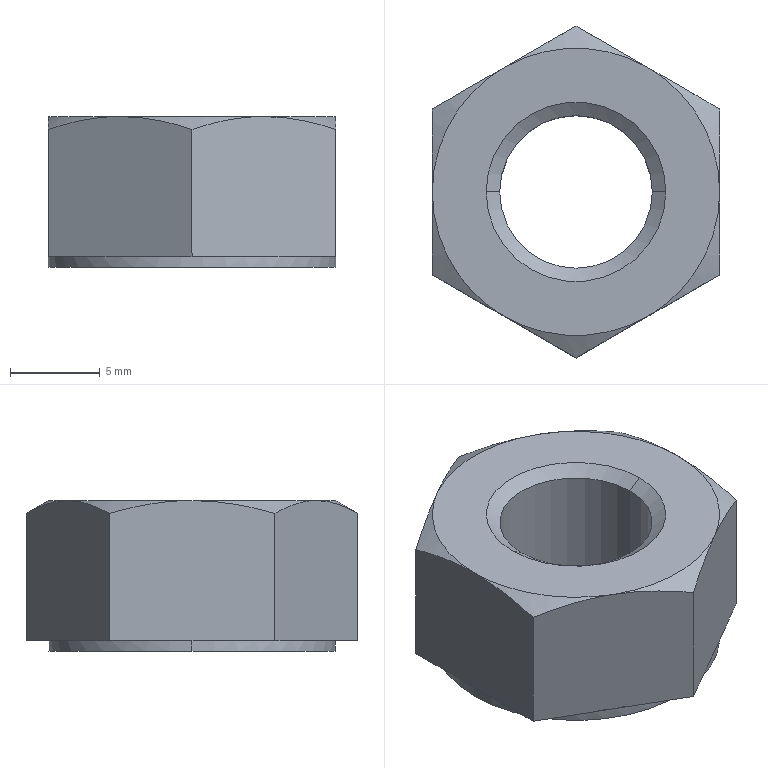Part | STEP file | hex nut style 1 gradeab_iso_ISO - 4032 - M10 - W - N | 1 solid | 30 faces | box 16 x 18.475 x 8.4 mm | volume 1357 mm3 | plane 14 | cone 10 | cylinder 6 | commonest cylinder face diameters 8.5 x2 10 x2 16 x2
STEP:
#1=CARTESIAN_POINT('',(5.,0.,-8.4));
#2=VERTEX_POINT('',#1);
#3=CARTESIAN_POINT('',(-5.,0.,-8.4));
#4=VERTEX_POINT('',#3);
#5=CARTESIAN_POINT('',(0.,0.,-8.4));
#6=DIRECTION('',(0.,0.,-1.));
#7=DIRECTION('',(1.,0.,0.));
#8=AXIS2_PLACEMENT_3D('',#5,#6,#7);
#9=CIRCLE('',#8,5.);
#10=EDGE_CURVE('',#2,#4,#9,.T.);
#11=ORIENTED_EDGE('',*,*,#10,.T.);
#12=CARTESIAN_POINT('',(-5.,0.,-8.375));
#13=VERTEX_POINT('',#12);
#14=CARTESIAN_POINT('',(-5.,0.,-25.038));
#15=DIRECTION('',(0.,0.,1.));
#16=VECTOR('',#15,1000.);
#17=LINE('',#14,#16);
#18=EDGE_CURVE('',#4,#13,#17,.T.);
#19=ORIENTED_EDGE('',*,*,#18,.T.);
#20=CARTESIAN_POINT('',(5.,0.,-8.375));
#21=VERTEX_POINT('',#20);
#22=CARTESIAN_POINT('',(0.,0.,-8.375));
#23=DIRECTION('',(0.,0.,1.));
#24=DIRECTION('',(1.,0.,0.));
#25=AXIS2_PLACEMENT_3D('',#22,#23,#24);
#26=CIRCLE('',#25,5.);
#27=EDGE_CURVE('',#13,#21,#26,.T.);
#28=ORIENTED_EDGE('',*,*,#27,.T.);
#29=CARTESIAN_POINT('',(5.,0.,-25.038));
#30=DIRECTION('',(0.,0.,1.));
#31=VECTOR('',#30,1000.);
#32=LINE('',#29,#31);
#33=EDGE_CURVE('',#2,#21,#32,.T.);
#34=ORIENTED_EDGE('',*,*,#33,.F.);
#35=EDGE_LOOP('',(#11,#19,#28,#34));
#36=FACE_OUTER_BOUND('',#35,.T.);
#37=CARTESIAN_POINT('',(0.,0.,-25.038));
#38=DIRECTION('',(0.,0.,1.));
#39=DIRECTION('',(1.,0.,0.));
#40=AXIS2_PLACEMENT_3D('',#37,#38,#39);
#41=CYLINDRICAL_SURFACE('',#40,5.);
#42=ADVANCED_FACE('',(#36),#41,.F.);
#43=CARTESIAN_POINT('',(-4.25,0.,-7.849));
#44=VERTEX_POINT('',#43);
#45=CARTESIAN_POINT('',(4.25,0.,-7.849));
#46=VERTEX_POINT('',#45);
#47=CARTESIAN_POINT('',(0.,0.,-7.849));
#48=DIRECTION('',(0.,0.,1.));
#49=DIRECTION('',(-1.,0.,0.));
#50=AXIS2_PLACEMENT_3D('',#47,#48,#49);
#51=CIRCLE('',#50,4.25);
#52=EDGE_CURVE('',#44,#46,#51,.T.);
#53=ORIENTED_EDGE('',*,*,#52,.T.);
#54=CARTESIAN_POINT('',(5.,0.,-8.375));
#55=DIRECTION('',(0.8192,0.,-0.5736));
#56=VECTOR('',#55,1000.);
#57=LINE('',#54,#56);
#58=EDGE_CURVE('',#46,#21,#57,.T.);
#59=ORIENTED_EDGE('',*,*,#58,.T.);
#60=ORIENTED_EDGE('',*,*,#27,.F.);
#61=CARTESIAN_POINT('',(-5.,0.,-8.375));
#62=DIRECTION('',(-0.8192,0.,-0.5736));
#63=VECTOR('',#62,1000.);
#64=LINE('',#61,#63);
#65=EDGE_CURVE('',#44,#13,#64,.T.);
#66=ORIENTED_EDGE('',*,*,#65,.F.);
#67=EDGE_LOOP('',(#53,#59,#60,#66));
#68=FACE_OUTER_BOUND('',#67,.T.);
#69=CARTESIAN_POINT('',(0.,0.,-8.375));
#70=DIRECTION('',(0.,0.,-1.));
#71=DIRECTION('',(-1.,0.,0.));
#72=AXIS2_PLACEMENT_3D('',#69,#70,#71);
#73=CONICAL_SURFACE('',#72,5.,0.9599);
#74=ADVANCED_FACE('',(#68),#73,.F.);
#75=CARTESIAN_POINT('',(4.25,0.,-0.5252));
#76=VERTEX_POINT('',#75);
#77=CARTESIAN_POINT('',(-4.25,0.,-0.5252));
#78=VERTEX_POINT('',#77);
#79=CARTESIAN_POINT('',(0.,0.,-0.5252));
#80=DIRECTION('',(0.,0.,-1.));
#81=DIRECTION('',(1.,0.,0.));
#82=AXIS2_PLACEMENT_3D('',#79,#80,#81);
#83=CIRCLE('',#82,4.25);
#84=EDGE_CURVE('',#76,#78,#83,.T.);
#85=ORIENTED_EDGE('',*,*,#84,.T.);
#86=CARTESIAN_POINT('',(-5.,0.,0.));
#87=VERTEX_POINT('',#86);
#88=CARTESIAN_POINT('',(-4.175,0.,-0.5777));
#89=DIRECTION('',(-0.8192,0.,0.5736));
#90=VECTOR('',#89,1000.);
#91=LINE('',#88,#90);
#92=EDGE_CURVE('',#78,#87,#91,.T.);
#93=ORIENTED_EDGE('',*,*,#92,.T.);
#94=CARTESIAN_POINT('',(5.,0.,0.));
#95=VERTEX_POINT('',#94);
#96=CARTESIAN_POINT('',(0.,0.,0.));
#97=DIRECTION('',(0.,0.,1.));
#98=DIRECTION('',(1.,0.,0.));
#99=AXIS2_PLACEMENT_3D('',#96,#97,#98);
#100=CIRCLE('',#99,5.);
#101=EDGE_CURVE('',#87,#95,#100,.T.);
#102=ORIENTED_EDGE('',*,*,#101,.T.);
#103=CARTESIAN_POINT('',(4.175,0.,-0.5777));
#104=DIRECTION('',(0.8192,0.,0.5736));
#105=VECTOR('',#104,1000.);
#106=LINE('',#103,#105);
#107=EDGE_CURVE('',#76,#95,#106,.T.);
#108=ORIENTED_EDGE('',*,*,#107,.F.);
#109=EDGE_LOOP('',(#85,#93,#102,#108));
#110=FACE_OUTER_BOUND('',#109,.T.);
#111=CARTESIAN_POINT('',(0.,0.,-0.5777));
#112=DIRECTION('',(0.,0.,1.));
#113=DIRECTION('',(1.,0.,0.));
#114=AXIS2_PLACEMENT_3D('',#111,#112,#113);
#115=CONICAL_SURFACE('',#114,4.175,0.9599);
#116=ADVANCED_FACE('',(#110),#115,.F.);
#117=CARTESIAN_POINT('',(-8.,0.,-8.4));
#118=VERTEX_POINT('',#117);
#119=CARTESIAN_POINT('',(8.,0.,-8.4));
#120=VERTEX_POINT('',#119);
#121=CARTESIAN_POINT('',(0.,0.,-8.4));
#122=DIRECTION('',(0.,0.,-1.));
#123=DIRECTION('',(1.,0.,0.));
#124=AXIS2_PLACEMENT_3D('',#121,#122,#123);
#125=CIRCLE('',#124,8.);
#126=EDGE_CURVE('',#118,#120,#125,.T.);
#127=ORIENTED_EDGE('',*,*,#126,.F.);
#128=CARTESIAN_POINT('',(-8.,0.,-7.8));
#129=VERTEX_POINT('',#128);
#130=CARTESIAN_POINT('',(-8.,0.,0.));
#131=DIRECTION('',(0.,0.,1.));
#132=VECTOR('',#131,1000.);
#133=LINE('',#130,#132);
#134=EDGE_CURVE('',#118,#129,#133,.T.);
#135=ORIENTED_EDGE('',*,*,#134,.T.);
#136=CARTESIAN_POINT('',(-4.,6.928,-7.8));
#137=VERTEX_POINT('',#136);
#138=CARTESIAN_POINT('',(0.,0.,-7.8));
#139=DIRECTION('',(0.,0.,1.));
#140=DIRECTION('',(1.,0.,0.));
#141=AXIS2_PLACEMENT_3D('',#138,#139,#140);
#142=CIRCLE('',#141,8.);
#143=EDGE_CURVE('',#137,#129,#142,.T.);
#144=ORIENTED_EDGE('',*,*,#143,.F.);
#145=CARTESIAN_POINT('',(4.,6.928,-7.8));
#146=VERTEX_POINT('',#145);
#147=CARTESIAN_POINT('',(0.,0.,-7.8));
#148=DIRECTION('',(0.,0.,1.));
#149=DIRECTION('',(1.,0.,0.));
#150=AXIS2_PLACEMENT_3D('',#147,#148,#149);
#151=CIRCLE('',#150,8.);
#152=EDGE_CURVE('',#146,#137,#151,.T.);
#153=ORIENTED_EDGE('',*,*,#152,.F.);
#154=CARTESIAN_POINT('',(8.,0.,-7.8));
#155=VERTEX_POINT('',#154);
#156=CARTESIAN_POINT('',(0.,0.,-7.8));
#157=DIRECTION('',(0.,0.,1.));
#158=DIRECTION('',(1.,0.,0.));
#159=AXIS2_PLACEMENT_3D('',#156,#157,#158);
#160=CIRCLE('',#159,8.);
#161=EDGE_CURVE('',#155,#146,#160,.T.);
#162=ORIENTED_EDGE('',*,*,#161,.F.);
#163=CARTESIAN_POINT('',(8.,0.,0.));
#164=DIRECTION('',(0.,0.,1.));
#165=VECTOR('',#164,1000.);
#166=LINE('',#163,#165);
#167=EDGE_CURVE('',#120,#155,#166,.T.);
#168=ORIENTED_EDGE('',*,*,#167,.F.);
#169=EDGE_LOOP('',(#127,#135,#144,#153,#162,#168));
#170=FACE_OUTER_BOUND('',#169,.T.);
#171=CARTESIAN_POINT('',(0.,0.,0.));
#172=DIRECTION('',(0.,0.,1.));
#173=DIRECTION('',(1.,0.,0.));
#174=AXIS2_PLACEMENT_3D('',#171,#172,#173);
#175=CYLINDRICAL_SURFACE('',#174,8.);
#176=ADVANCED_FACE('',(#170),#175,.T.);
#177=ORIENTED_EDGE('',*,*,#52,.F.);
#178=CARTESIAN_POINT('',(-4.25,0.,-8.4));
#179=DIRECTION('',(0.,0.,1.));
#180=VECTOR('',#179,1000.);
#181=LINE('',#178,#180);
#182=EDGE_CURVE('',#44,#78,#181,.T.);
#183=ORIENTED_EDGE('',*,*,#182,.T.);
#184=ORIENTED_EDGE('',*,*,#84,.F.);
#185=CARTESIAN_POINT('',(4.25,0.,-8.4));
#186=DIRECTION('',(0.,0.,1.));
#187=VECTOR('',#186,1000.);
#188=LINE('',#185,#187);
#189=EDGE_CURVE('',#46,#76,#188,.T.);
#190=ORIENTED_EDGE('',*,*,#189,.F.);
#191=EDGE_LOOP('',(#177,#183,#184,#190));
#192=FACE_OUTER_BOUND('',#191,.T.);
#193=CARTESIAN_POINT('',(0.,0.,-8.4));
#194=DIRECTION('',(0.,0.,1.));
#195=DIRECTION('',(1.,0.,0.));
#196=AXIS2_PLACEMENT_3D('',#193,#194,#195);
#197=CYLINDRICAL_SURFACE('',#196,4.25);
#198=ADVANCED_FACE('',(#192),#197,.F.);
#199=ORIENTED_EDGE('',*,*,#182,.F.);
#200=CARTESIAN_POINT('',(0.,0.,-7.849));
#201=DIRECTION('',(0.,0.,1.));
#202=DIRECTION('',(-1.,0.,0.));
#203=AXIS2_PLACEMENT_3D('',#200,#201,#202);
#204=CIRCLE('',#203,4.25);
#205=EDGE_CURVE('',#46,#44,#204,.T.);
#206=ORIENTED_EDGE('',*,*,#205,.F.);
#207=ORIENTED_EDGE('',*,*,#189,.T.);
#208=CARTESIAN_POINT('',(0.,0.,-0.5252));
#209=DIRECTION('',(0.,0.,-1.));
#210=DIRECTION('',(1.,0.,0.));
#211=AXIS2_PLACEMENT_3D('',#208,#209,#210);
#212=CIRCLE('',#211,4.25);
#213=EDGE_CURVE('',#78,#76,#212,.T.);
#214=ORIENTED_EDGE('',*,*,#213,.F.);
#215=EDGE_LOOP('',(#199,#206,#207,#214));
#216=FACE_OUTER_BOUND('',#215,.T.);
#217=CARTESIAN_POINT('',(0.,0.,-8.4));
#218=DIRECTION('',(0.,0.,1.));
#219=DIRECTION('',(1.,0.,0.));
#220=AXIS2_PLACEMENT_3D('',#217,#218,#219);
#221=CYLINDRICAL_SURFACE('',#220,4.25);
#222=ADVANCED_FACE('',(#216),#221,.F.);
#223=CARTESIAN_POINT('',(-8.,4.619,-7.8));
#224=VERTEX_POINT('',#223);
#225=CARTESIAN_POINT('',(-8.,4.619,-0.7145));
#226=VERTEX_POINT('',#225);
#227=CARTESIAN_POINT('',(-8.,4.619,-8.4));
#228=DIRECTION('',(0.,0.,1.));
#229=VECTOR('',#228,1000.);
#230=LINE('',#227,#229);
#231=EDGE_CURVE('',#224,#226,#230,.T.);
#232=ORIENTED_EDGE('',*,*,#231,.T.);
#233=CARTESIAN_POINT('',(-4.,6.928,0.));
#234=VERTEX_POINT('',#233);
#235=CARTESIAN_POINT('',(-8.,4.619,-0.7145));
#236=CARTESIAN_POINT('',(-7.346,4.997,-0.4964));
#237=CARTESIAN_POINT('',(-6.687,5.377,-0.3167));
#238=CARTESIAN_POINT('',(-5.354,6.146,-0.0681));
#239=CARTESIAN_POINT('',(-4.681,6.535,0.));
#240=CARTESIAN_POINT('',(-4.,6.928,0.));
#241=B_SPLINE_CURVE_WITH_KNOTS('',3,(#235,#236,#237,#238,#239,#240),.UNSPECIFIED.,.F.,.F.,(4,2,4),(0.000000238,0.002337,0.004674),.UNSPECIFIED.);
#242=EDGE_CURVE('',#226,#234,#241,.T.);
#243=ORIENTED_EDGE('',*,*,#242,.T.);
#244=CARTESIAN_POINT('',(0.,9.238,-0.7145));
#245=VERTEX_POINT('',#244);
#246=CARTESIAN_POINT('',(-4.,6.928,0.));
#247=CARTESIAN_POINT('',(-3.661,7.124,0.));
#248=CARTESIAN_POINT('',(-3.32,7.321,-0.01689));
#249=CARTESIAN_POINT('',(-2.645,7.711,-0.08225));
#250=CARTESIAN_POINT('',(-2.31,7.904,-0.1307));
#251=CARTESIAN_POINT('',(-1.311,8.481,-0.3174));
#252=CARTESIAN_POINT('',(-0.6527,8.861,-0.497));
#253=CARTESIAN_POINT('',(0.,9.238,-0.7145));
#254=B_SPLINE_CURVE_WITH_KNOTS('',3,(#246,#247,#248,#249,#250,#251,#252,#253),.UNSPECIFIED.,.F.,.F.,(4,2,2,4),(0.004674,0.005838,0.007002,0.00933),.UNSPECIFIED.);
#255=EDGE_CURVE('',#234,#245,#254,.T.);
#256=ORIENTED_EDGE('',*,*,#255,.T.);
#257=CARTESIAN_POINT('',(0.,9.238,-7.8));
#258=VERTEX_POINT('',#257);
#259=CARTESIAN_POINT('',(0.,9.238,-8.4));
#260=DIRECTION('',(0.,0.,1.));
#261=VECTOR('',#260,1000.);
#262=LINE('',#259,#261);
#263=EDGE_CURVE('',#258,#245,#262,.T.);
#264=ORIENTED_EDGE('',*,*,#263,.F.);
#265=CARTESIAN_POINT('',(0.,9.238,-7.8));
#266=DIRECTION('',(-0.866,-0.5,0.));
#267=VECTOR('',#266,1000.);
#268=LINE('',#265,#267);
#269=EDGE_CURVE('',#258,#137,#268,.T.);
#270=ORIENTED_EDGE('',*,*,#269,.T.);
#271=CARTESIAN_POINT('',(0.,9.238,-7.8));
#272=DIRECTION('',(-0.866,-0.5,0.));
#273=VECTOR('',#272,1000.);
#274=LINE('',#271,#273);
#275=EDGE_CURVE('',#137,#224,#274,.T.);
#276=ORIENTED_EDGE('',*,*,#275,.T.);
#277=EDGE_LOOP('',(#232,#243,#256,#264,#270,#276));
#278=FACE_OUTER_BOUND('',#277,.T.);
#279=CARTESIAN_POINT('',(0.,9.238,-8.4));
#280=DIRECTION('',(-0.5,0.866,0.));
#281=DIRECTION('',(-0.866,-0.5,0.));
#282=AXIS2_PLACEMENT_3D('',#279,#280,#281);
#283=PLANE('',#282);
#284=ADVANCED_FACE('',(#278),#283,.T.);
#285=ORIENTED_EDGE('',*,*,#263,.T.);
#286=CARTESIAN_POINT('',(4.,6.928,0.));
#287=VERTEX_POINT('',#286);
#288=CARTESIAN_POINT('',(0.,9.238,-0.7145));
#289=CARTESIAN_POINT('',(0.6543,8.86,-0.4964));
#290=CARTESIAN_POINT('',(1.313,8.479,-0.3167));
#291=CARTESIAN_POINT('',(2.646,7.71,-0.0681));
#292=CARTESIAN_POINT('',(3.319,7.322,0.));
#293=CARTESIAN_POINT('',(4.,6.928,0.));
#294=B_SPLINE_CURVE_WITH_KNOTS('',3,(#288,#289,#290,#291,#292,#293),.UNSPECIFIED.,.F.,.F.,(4,2,4),(0.000000238,0.002337,0.004674),.UNSPECIFIED.);
#295=EDGE_CURVE('',#245,#287,#294,.T.);
#296=ORIENTED_EDGE('',*,*,#295,.T.);
#297=CARTESIAN_POINT('',(8.,4.619,-0.7145));
#298=VERTEX_POINT('',#297);
#299=CARTESIAN_POINT('',(4.,6.928,0.));
#300=CARTESIAN_POINT('',(4.339,6.732,0.));
#301=CARTESIAN_POINT('',(4.68,6.535,-0.01689));
#302=CARTESIAN_POINT('',(5.355,6.146,-0.08225));
#303=CARTESIAN_POINT('',(5.69,5.952,-0.1307));
#304=CARTESIAN_POINT('',(6.689,5.376,-0.3174));
#305=CARTESIAN_POINT('',(7.347,4.996,-0.497));
#306=CARTESIAN_POINT('',(8.,4.619,-0.7145));
#307=B_SPLINE_CURVE_WITH_KNOTS('',3,(#299,#300,#301,#302,#303,#304,#305,#306),.UNSPECIFIED.,.F.,.F.,(4,2,2,4),(0.004674,0.005838,0.007002,0.00933),.UNSPECIFIED.);
#308=EDGE_CURVE('',#287,#298,#307,.T.);
#309=ORIENTED_EDGE('',*,*,#308,.T.);
#310=CARTESIAN_POINT('',(8.,4.619,-7.8));
#311=VERTEX_POINT('',#310);
#312=CARTESIAN_POINT('',(8.,4.619,-8.4));
#313=DIRECTION('',(0.,0.,1.));
#314=VECTOR('',#313,1000.);
#315=LINE('',#312,#314);
#316=EDGE_CURVE('',#311,#298,#315,.T.);
#317=ORIENTED_EDGE('',*,*,#316,.F.);
#318=CARTESIAN_POINT('',(8.,4.619,-7.8));
#319=DIRECTION('',(-0.866,0.5,0.));
#320=VECTOR('',#319,1000.);
#321=LINE('',#318,#320);
#322=EDGE_CURVE('',#311,#146,#321,.T.);
#323=ORIENTED_EDGE('',*,*,#322,.T.);
#324=CARTESIAN_POINT('',(8.,4.619,-7.8));
#325=DIRECTION('',(-0.866,0.5,0.));
#326=VECTOR('',#325,1000.);
#327=LINE('',#324,#326);
#328=EDGE_CURVE('',#146,#258,#327,.T.);
#329=ORIENTED_EDGE('',*,*,#328,.T.);
#330=EDGE_LOOP('',(#285,#296,#309,#317,#323,#329));
#331=FACE_OUTER_BOUND('',#330,.T.);
#332=CARTESIAN_POINT('',(8.,4.619,-8.4));
#333=DIRECTION('',(0.5,0.866,0.));
#334=DIRECTION('',(-0.866,0.5,0.));
#335=AXIS2_PLACEMENT_3D('',#332,#333,#334);
#336=PLANE('',#335);
#337=ADVANCED_FACE('',(#331),#336,.T.);
#338=CARTESIAN_POINT('',(8.,-4.619,-0.7145));
#339=VERTEX_POINT('',#338);
#340=CARTESIAN_POINT('',(8.,0.,0.));
#341=VERTEX_POINT('',#340);
#342=CARTESIAN_POINT('',(8.,-4.619,-0.7145));
#343=CARTESIAN_POINT('',(8.,-3.868,-0.4977));
#344=CARTESIAN_POINT('',(8.,-3.098,-0.3158));
#345=CARTESIAN_POINT('',(8.,-1.556,-0.06709));
#346=CARTESIAN_POINT('',(8.,-0.7805,0.));
#347=CARTESIAN_POINT('',(8.,0.,0.));
#348=B_SPLINE_CURVE_WITH_KNOTS('',3,(#342,#343,#344,#345,#346,#347),.UNSPECIFIED.,.F.,.F.,(4,2,4),(0.008241,0.01058,0.01291),.UNSPECIFIED.);
#349=EDGE_CURVE('',#339,#341,#348,.T.);
#350=ORIENTED_EDGE('',*,*,#349,.F.);
#351=CARTESIAN_POINT('',(8.,-4.619,-7.8));
#352=VERTEX_POINT('',#351);
#353=CARTESIAN_POINT('',(8.,-4.619,-8.4));
#354=DIRECTION('',(0.,0.,1.));
#355=VECTOR('',#354,1000.);
#356=LINE('',#353,#355);
#357=EDGE_CURVE('',#352,#339,#356,.T.);
#358=ORIENTED_EDGE('',*,*,#357,.F.);
#359=CARTESIAN_POINT('',(8.,4.619,-7.8));
#360=DIRECTION('',(0.,-1.,0.));
#361=VECTOR('',#360,1000.);
#362=LINE('',#359,#361);
#363=EDGE_CURVE('',#155,#352,#362,.T.);
#364=ORIENTED_EDGE('',*,*,#363,.F.);
#365=CARTESIAN_POINT('',(8.,4.619,-7.8));
#366=DIRECTION('',(0.,-1.,0.));
#367=VECTOR('',#366,1000.);
#368=LINE('',#365,#367);
#369=EDGE_CURVE('',#311,#155,#368,.T.);
#370=ORIENTED_EDGE('',*,*,#369,.F.);
#371=ORIENTED_EDGE('',*,*,#316,.T.);
#372=CARTESIAN_POINT('',(8.,0.,0.));
#373=CARTESIAN_POINT('',(8.,0.781,0.));
#374=CARTESIAN_POINT('',(8.,1.573,-0.06894));
#375=CARTESIAN_POINT('',(8.,3.115,-0.3194));
#376=CARTESIAN_POINT('',(8.,3.872,-0.4989));
#377=CARTESIAN_POINT('',(8.,4.619,-0.7145));
#378=B_SPLINE_CURVE_WITH_KNOTS('',3,(#372,#373,#374,#375,#376,#377),.UNSPECIFIED.,.F.,.F.,(4,2,4),(0.01291,0.01525,0.01759),.UNSPECIFIED.);
#379=EDGE_CURVE('',#341,#298,#378,.T.);
#380=ORIENTED_EDGE('',*,*,#379,.F.);
#381=EDGE_LOOP('',(#350,#358,#364,#370,#371,#380));
#382=FACE_OUTER_BOUND('',#381,.T.);
#383=CARTESIAN_POINT('',(8.,4.619,-8.4));
#384=DIRECTION('',(-1.,0.,0.));
#385=DIRECTION('',(0.,0.,1.));
#386=AXIS2_PLACEMENT_3D('',#383,#384,#385);
#387=PLANE('',#386);
#388=ADVANCED_FACE('',(#382),#387,.F.);
#389=ORIENTED_EDGE('',*,*,#357,.T.);
#390=CARTESIAN_POINT('',(4.,-6.928,0.));
#391=VERTEX_POINT('',#390);
#392=CARTESIAN_POINT('',(8.,-4.619,-0.7145));
#393=CARTESIAN_POINT('',(7.346,-4.997,-0.4964));
#394=CARTESIAN_POINT('',(6.687,-5.377,-0.3167));
#395=CARTESIAN_POINT('',(5.354,-6.146,-0.0681));
#396=CARTESIAN_POINT('',(4.681,-6.535,0.));
#397=CARTESIAN_POINT('',(4.,-6.928,0.));
#398=B_SPLINE_CURVE_WITH_KNOTS('',3,(#392,#393,#394,#395,#396,#397),.UNSPECIFIED.,.F.,.F.,(4,2,4),(0.000000238,0.002337,0.004674),.UNSPECIFIED.);
#399=EDGE_CURVE('',#339,#391,#398,.T.);
#400=ORIENTED_EDGE('',*,*,#399,.T.);
#401=CARTESIAN_POINT('',(0.,-9.238,-0.7145));
#402=VERTEX_POINT('',#401);
#403=CARTESIAN_POINT('',(4.,-6.928,0.));
#404=CARTESIAN_POINT('',(3.661,-7.124,0.));
#405=CARTESIAN_POINT('',(3.32,-7.321,-0.01689));
#406=CARTESIAN_POINT('',(2.645,-7.711,-0.08225));
#407=CARTESIAN_POINT('',(2.31,-7.904,-0.1307));
#408=CARTESIAN_POINT('',(1.311,-8.481,-0.3174));
#409=CARTESIAN_POINT('',(0.6527,-8.861,-0.497));
#410=CARTESIAN_POINT('',(0.,-9.238,-0.7145));
#411=B_SPLINE_CURVE_WITH_KNOTS('',3,(#403,#404,#405,#406,#407,#408,#409,#410),.UNSPECIFIED.,.F.,.F.,(4,2,2,4),(0.004674,0.005838,0.007002,0.00933),.UNSPECIFIED.);
#412=EDGE_CURVE('',#391,#402,#411,.T.);
#413=ORIENTED_EDGE('',*,*,#412,.T.);
#414=CARTESIAN_POINT('',(0.,-9.238,-7.8));
#415=VERTEX_POINT('',#414);
#416=CARTESIAN_POINT('',(0.,-9.238,-8.4));
#417=DIRECTION('',(0.,0.,1.));
#418=VECTOR('',#417,1000.);
#419=LINE('',#416,#418);
#420=EDGE_CURVE('',#415,#402,#419,.T.);
#421=ORIENTED_EDGE('',*,*,#420,.F.);
#422=CARTESIAN_POINT('',(4.,-6.928,-7.8));
#423=VERTEX_POINT('',#422);
#424=CARTESIAN_POINT('',(0.,-9.238,-7.8));
#425=DIRECTION('',(0.866,0.5,0.));
#426=VECTOR('',#425,1000.);
#427=LINE('',#424,#426);
#428=EDGE_CURVE('',#415,#423,#427,.T.);
#429=ORIENTED_EDGE('',*,*,#428,.T.);
#430=CARTESIAN_POINT('',(0.,-9.238,-7.8));
#431=DIRECTION('',(0.866,0.5,0.));
#432=VECTOR('',#431,1000.);
#433=LINE('',#430,#432);
#434=EDGE_CURVE('',#423,#352,#433,.T.);
#435=ORIENTED_EDGE('',*,*,#434,.T.);
#436=EDGE_LOOP('',(#389,#400,#413,#421,#429,#435));
#437=FACE_OUTER_BOUND('',#436,.T.);
#438=CARTESIAN_POINT('',(0.,-9.238,-8.4));
#439=DIRECTION('',(0.5,-0.866,0.));
#440=DIRECTION('',(0.866,0.5,0.));
#441=AXIS2_PLACEMENT_3D('',#438,#439,#440);
#442=PLANE('',#441);
#443=ADVANCED_FACE('',(#437),#442,.T.);
#444=ORIENTED_EDGE('',*,*,#420,.T.);
#445=CARTESIAN_POINT('',(-4.,-6.928,0.));
#446=VERTEX_POINT('',#445);
#447=CARTESIAN_POINT('',(0.,-9.238,-0.7145));
#448=CARTESIAN_POINT('',(-0.6543,-8.86,-0.4964));
#449=CARTESIAN_POINT('',(-1.313,-8.479,-0.3167));
#450=CARTESIAN_POINT('',(-2.646,-7.71,-0.0681));
#451=CARTESIAN_POINT('',(-3.319,-7.322,0.));
#452=CARTESIAN_POINT('',(-4.,-6.928,0.));
#453=B_SPLINE_CURVE_WITH_KNOTS('',3,(#447,#448,#449,#450,#451,#452),.UNSPECIFIED.,.F.,.F.,(4,2,4),(0.000000238,0.002337,0.004674),.UNSPECIFIED.);
#454=EDGE_CURVE('',#402,#446,#453,.T.);
#455=ORIENTED_EDGE('',*,*,#454,.T.);
#456=CARTESIAN_POINT('',(-8.,-4.619,-0.7145));
#457=VERTEX_POINT('',#456);
#458=CARTESIAN_POINT('',(-4.,-6.928,0.));
#459=CARTESIAN_POINT('',(-4.339,-6.732,0.));
#460=CARTESIAN_POINT('',(-4.68,-6.535,-0.01689));
#461=CARTESIAN_POINT('',(-5.355,-6.146,-0.08225));
#462=CARTESIAN_POINT('',(-5.69,-5.952,-0.1307));
#463=CARTESIAN_POINT('',(-6.689,-5.376,-0.3174));
#464=CARTESIAN_POINT('',(-7.347,-4.996,-0.497));
#465=CARTESIAN_POINT('',(-8.,-4.619,-0.7145));
#466=B_SPLINE_CURVE_WITH_KNOTS('',3,(#458,#459,#460,#461,#462,#463,#464,#465),.UNSPECIFIED.,.F.,.F.,(4,2,2,4),(0.004674,0.005838,0.007002,0.00933),.UNSPECIFIED.);
#467=EDGE_CURVE('',#446,#457,#466,.T.);
#468=ORIENTED_EDGE('',*,*,#467,.T.);
#469=CARTESIAN_POINT('',(-8.,-4.619,-7.8));
#470=VERTEX_POINT('',#469);
#471=CARTESIAN_POINT('',(-8.,-4.619,-8.4));
#472=DIRECTION('',(0.,0.,1.));
#473=VECTOR('',#472,1000.);
#474=LINE('',#471,#473);
#475=EDGE_CURVE('',#470,#457,#474,.T.);
#476=ORIENTED_EDGE('',*,*,#475,.F.);
#477=CARTESIAN_POINT('',(-4.,-6.928,-7.8));
#478=VERTEX_POINT('',#477);
#479=CARTESIAN_POINT('',(-8.,-4.619,-7.8));
#480=DIRECTION('',(0.866,-0.5,0.));
#481=VECTOR('',#480,1000.);
#482=LINE('',#479,#481);
#483=EDGE_CURVE('',#470,#478,#482,.T.);
#484=ORIENTED_EDGE('',*,*,#483,.T.);
#485=CARTESIAN_POINT('',(-8.,-4.619,-7.8));
#486=DIRECTION('',(0.866,-0.5,0.));
#487=VECTOR('',#486,1000.);
#488=LINE('',#485,#487);
#489=EDGE_CURVE('',#478,#415,#488,.T.);
#490=ORIENTED_EDGE('',*,*,#489,.T.);
#491=EDGE_LOOP('',(#444,#455,#468,#476,#484,#490));
#492=FACE_OUTER_BOUND('',#491,.T.);
#493=CARTESIAN_POINT('',(-8.,-4.619,-8.4));
#494=DIRECTION('',(-0.5,-0.866,0.));
#495=DIRECTION('',(0.866,-0.5,0.));
#496=AXIS2_PLACEMENT_3D('',#493,#494,#495);
#497=PLANE('',#496);
#498=ADVANCED_FACE('',(#492),#497,.T.);
#499=ORIENTED_EDGE('',*,*,#475,.T.);
#500=CARTESIAN_POINT('',(-8.,0.,0.));
#501=VERTEX_POINT('',#500);
#502=CARTESIAN_POINT('',(-8.,-4.619,-0.7145));
#503=CARTESIAN_POINT('',(-8.,-3.868,-0.4977));
#504=CARTESIAN_POINT('',(-8.,-3.098,-0.3158));
#505=CARTESIAN_POINT('',(-8.,-1.556,-0.06709));
#506=CARTESIAN_POINT('',(-8.,-0.7805,0.));
#507=CARTESIAN_POINT('',(-8.,0.,0.));
#508=B_SPLINE_CURVE_WITH_KNOTS('',3,(#502,#503,#504,#505,#506,#507),.UNSPECIFIED.,.F.,.F.,(4,2,4),(0.008241,0.01058,0.01291),.UNSPECIFIED.);
#509=EDGE_CURVE('',#457,#501,#508,.T.);
#510=ORIENTED_EDGE('',*,*,#509,.T.);
#511=CARTESIAN_POINT('',(-8.,0.,0.));
#512=CARTESIAN_POINT('',(-8.,0.781,0.));
#513=CARTESIAN_POINT('',(-8.,1.573,-0.06894));
#514=CARTESIAN_POINT('',(-8.,3.115,-0.3194));
#515=CARTESIAN_POINT('',(-8.,3.872,-0.4989));
#516=CARTESIAN_POINT('',(-8.,4.619,-0.7145));
#517=B_SPLINE_CURVE_WITH_KNOTS('',3,(#511,#512,#513,#514,#515,#516),.UNSPECIFIED.,.F.,.F.,(4,2,4),(0.01291,0.01525,0.01759),.UNSPECIFIED.);
#518=EDGE_CURVE('',#501,#226,#517,.T.);
#519=ORIENTED_EDGE('',*,*,#518,.T.);
#520=ORIENTED_EDGE('',*,*,#231,.F.);
#521=CARTESIAN_POINT('',(-8.,4.619,-7.8));
#522=DIRECTION('',(0.,-1.,0.));
#523=VECTOR('',#522,1000.);
#524=LINE('',#521,#523);
#525=EDGE_CURVE('',#224,#129,#524,.T.);
#526=ORIENTED_EDGE('',*,*,#525,.T.);
#527=CARTESIAN_POINT('',(-8.,4.619,-7.8));
#528=DIRECTION('',(0.,-1.,0.));
#529=VECTOR('',#528,1000.);
#530=LINE('',#527,#529);
#531=EDGE_CURVE('',#129,#470,#530,.T.);
#532=ORIENTED_EDGE('',*,*,#531,.T.);
#533=EDGE_LOOP('',(#499,#510,#519,#520,#526,#532));
#534=FACE_OUTER_BOUND('',#533,.T.);
#535=CARTESIAN_POINT('',(-8.,4.619,-8.4));
#536=DIRECTION('',(-1.,0.,0.));
#537=DIRECTION('',(0.,0.,1.));
#538=AXIS2_PLACEMENT_3D('',#535,#536,#537);
#539=PLANE('',#538);
#540=ADVANCED_FACE('',(#534),#539,.T.);
#541=CARTESIAN_POINT('',(0.,0.,0.));
#542=DIRECTION('',(0.,0.,1.));
#543=DIRECTION('',(1.,0.,0.));
#544=AXIS2_PLACEMENT_3D('',#541,#542,#543);
#545=CIRCLE('',#544,5.);
#546=EDGE_CURVE('',#95,#87,#545,.T.);
#547=ORIENTED_EDGE('',*,*,#546,.F.);
#548=ORIENTED_EDGE('',*,*,#101,.F.);
#549=EDGE_LOOP('',(#547,#548));
#550=FACE_BOUND('',#549,.T.);
#551=CARTESIAN_POINT('',(0.,0.,0.));
#552=DIRECTION('',(0.,0.,-1.));
#553=DIRECTION('',(1.,0.,0.));
#554=AXIS2_PLACEMENT_3D('',#551,#552,#553);
#555=CIRCLE('',#554,8.);
#556=EDGE_CURVE('',#341,#391,#555,.T.);
#557=ORIENTED_EDGE('',*,*,#556,.F.);
#558=CARTESIAN_POINT('',(0.,0.,0.));
#559=DIRECTION('',(0.,0.,1.));
#560=DIRECTION('',(1.,0.,0.));
#561=AXIS2_PLACEMENT_3D('',#558,#559,#560);
#562=CIRCLE('',#561,8.);
#563=EDGE_CURVE('',#341,#287,#562,.T.);
#564=ORIENTED_EDGE('',*,*,#563,.T.);
#565=CARTESIAN_POINT('',(0.,0.,0.));
#566=DIRECTION('',(0.,0.,-1.));
#567=DIRECTION('',(1.,0.,0.));
#568=AXIS2_PLACEMENT_3D('',#565,#566,#567);
#569=CIRCLE('',#568,8.);
#570=EDGE_CURVE('',#234,#287,#569,.T.);
#571=ORIENTED_EDGE('',*,*,#570,.F.);
#572=CARTESIAN_POINT('',(0.,0.,0.));
#573=DIRECTION('',(0.,0.,-1.));
#574=DIRECTION('',(1.,0.,0.));
#575=AXIS2_PLACEMENT_3D('',#572,#573,#574);
#576=CIRCLE('',#575,8.);
#577=EDGE_CURVE('',#501,#234,#576,.T.);
#578=ORIENTED_EDGE('',*,*,#577,.F.);
#579=CARTESIAN_POINT('',(0.,0.,0.));
#580=DIRECTION('',(0.,0.,-1.));
#581=DIRECTION('',(1.,0.,0.));
#582=AXIS2_PLACEMENT_3D('',#579,#580,#581);
#583=CIRCLE('',#582,8.);
#584=EDGE_CURVE('',#446,#501,#583,.T.);
#585=ORIENTED_EDGE('',*,*,#584,.F.);
#586=CARTESIAN_POINT('',(0.,0.,0.));
#587=DIRECTION('',(0.,0.,-1.));
#588=DIRECTION('',(1.,0.,0.));
#589=AXIS2_PLACEMENT_3D('',#586,#587,#588);
#590=CIRCLE('',#589,8.);
#591=EDGE_CURVE('',#391,#446,#590,.T.);
#592=ORIENTED_EDGE('',*,*,#591,.F.);
#593=EDGE_LOOP('',(#557,#564,#571,#578,#585,#592));
#594=FACE_OUTER_BOUND('',#593,.T.);
#595=CARTESIAN_POINT('',(-16.,0.,0.));
#596=DIRECTION('',(0.,0.,1.));
#597=DIRECTION('',(1.,0.,0.));
#598=AXIS2_PLACEMENT_3D('',#595,#596,#597);
#599=PLANE('',#598);
#600=ADVANCED_FACE('',(#550,#594),#599,.T.);
#601=ORIENTED_EDGE('',*,*,#10,.F.);
#602=CARTESIAN_POINT('',(0.,0.,-8.4));
#603=DIRECTION('',(0.,0.,-1.));
#604=DIRECTION('',(1.,0.,0.));
#605=AXIS2_PLACEMENT_3D('',#602,#603,#604);
#606=CIRCLE('',#605,5.);
#607=EDGE_CURVE('',#4,#2,#606,.T.);
#608=ORIENTED_EDGE('',*,*,#607,.F.);
#609=EDGE_LOOP('',(#601,#608));
#610=FACE_BOUND('',#609,.T.);
#611=CARTESIAN_POINT('',(0.,0.,-8.4));
#612=DIRECTION('',(0.,0.,-1.));
#613=DIRECTION('',(1.,0.,0.));
#614=AXIS2_PLACEMENT_3D('',#611,#612,#613);
#615=CIRCLE('',#614,8.);
#616=EDGE_CURVE('',#120,#118,#615,.T.);
#617=ORIENTED_EDGE('',*,*,#616,.T.);
#618=ORIENTED_EDGE('',*,*,#126,.T.);
#619=EDGE_LOOP('',(#617,#618));
#620=FACE_OUTER_BOUND('',#619,.T.);
#621=CARTESIAN_POINT('',(-16.,0.,-8.4));
#622=DIRECTION('',(0.,0.,1.));
#623=DIRECTION('',(1.,0.,0.));
#624=AXIS2_PLACEMENT_3D('',#621,#622,#623);
#625=PLANE('',#624);
#626=ADVANCED_FACE('',(#610,#620),#625,.F.);
#627=ORIENTED_EDGE('',*,*,#369,.T.);
#628=ORIENTED_EDGE('',*,*,#161,.T.);
#629=ORIENTED_EDGE('',*,*,#322,.F.);
#630=EDGE_LOOP('',(#627,#628,#629));
#631=FACE_OUTER_BOUND('',#630,.T.);
#632=CARTESIAN_POINT('',(0.,19.238,-7.8));
#633=DIRECTION('',(0.,0.,-1.));
#634=DIRECTION('',(-1.,0.,0.));
#635=AXIS2_PLACEMENT_3D('',#632,#633,#634);
#636=PLANE('',#635);
#637=ADVANCED_FACE('',(#631),#636,.T.);
#638=ORIENTED_EDGE('',*,*,#363,.T.);
#639=ORIENTED_EDGE('',*,*,#434,.F.);
#640=CARTESIAN_POINT('',(0.,0.,-7.8));
#641=DIRECTION('',(0.,0.,1.));
#642=DIRECTION('',(1.,0.,0.));
#643=AXIS2_PLACEMENT_3D('',#640,#641,#642);
#644=CIRCLE('',#643,8.);
#645=EDGE_CURVE('',#423,#155,#644,.T.);
#646=ORIENTED_EDGE('',*,*,#645,.T.);
#647=EDGE_LOOP('',(#638,#639,#646));
#648=FACE_OUTER_BOUND('',#647,.T.);
#649=CARTESIAN_POINT('',(0.,19.238,-7.8));
#650=DIRECTION('',(0.,0.,-1.));
#651=DIRECTION('',(-1.,0.,0.));
#652=AXIS2_PLACEMENT_3D('',#649,#650,#651);
#653=PLANE('',#652);
#654=ADVANCED_FACE('',(#648),#653,.T.);
#655=ORIENTED_EDGE('',*,*,#152,.T.);
#656=ORIENTED_EDGE('',*,*,#269,.F.);
#657=ORIENTED_EDGE('',*,*,#328,.F.);
#658=EDGE_LOOP('',(#655,#656,#657));
#659=FACE_OUTER_BOUND('',#658,.T.);
#660=CARTESIAN_POINT('',(0.,19.238,-7.8));
#661=DIRECTION('',(0.,0.,-1.));
#662=DIRECTION('',(-1.,0.,0.));
#663=AXIS2_PLACEMENT_3D('',#660,#661,#662);
#664=PLANE('',#663);
#665=ADVANCED_FACE('',(#659),#664,.T.);
#666=ORIENTED_EDGE('',*,*,#489,.F.);
#667=CARTESIAN_POINT('',(0.,0.,-7.8));
#668=DIRECTION('',(0.,0.,1.));
#669=DIRECTION('',(1.,0.,0.));
#670=AXIS2_PLACEMENT_3D('',#667,#668,#669);
#671=CIRCLE('',#670,8.);
#672=EDGE_CURVE('',#478,#423,#671,.T.);
#673=ORIENTED_EDGE('',*,*,#672,.T.);
#674=ORIENTED_EDGE('',*,*,#428,.F.);
#675=EDGE_LOOP('',(#666,#673,#674));
#676=FACE_OUTER_BOUND('',#675,.T.);
#677=CARTESIAN_POINT('',(0.,19.238,-7.8));
#678=DIRECTION('',(0.,0.,-1.));
#679=DIRECTION('',(-1.,0.,0.));
#680=AXIS2_PLACEMENT_3D('',#677,#678,#679);
#681=PLANE('',#680);
#682=ADVANCED_FACE('',(#676),#681,.T.);
#683=ORIENTED_EDGE('',*,*,#143,.T.);
#684=ORIENTED_EDGE('',*,*,#525,.F.);
#685=ORIENTED_EDGE('',*,*,#275,.F.);
#686=EDGE_LOOP('',(#683,#684,#685));
#687=FACE_OUTER_BOUND('',#686,.T.);
#688=CARTESIAN_POINT('',(0.,19.238,-7.8));
#689=DIRECTION('',(0.,0.,-1.));
#690=DIRECTION('',(-1.,0.,0.));
#691=AXIS2_PLACEMENT_3D('',#688,#689,#690);
#692=PLANE('',#691);
#693=ADVANCED_FACE('',(#687),#692,.T.);
#694=ORIENTED_EDGE('',*,*,#134,.F.);
#695=ORIENTED_EDGE('',*,*,#616,.F.);
#696=ORIENTED_EDGE('',*,*,#167,.T.);
#697=ORIENTED_EDGE('',*,*,#645,.F.);
#698=ORIENTED_EDGE('',*,*,#672,.F.);
#699=CARTESIAN_POINT('',(0.,0.,-7.8));
#700=DIRECTION('',(0.,0.,1.));
#701=DIRECTION('',(1.,0.,0.));
#702=AXIS2_PLACEMENT_3D('',#699,#700,#701);
#703=CIRCLE('',#702,8.);
#704=EDGE_CURVE('',#129,#478,#703,.T.);
#705=ORIENTED_EDGE('',*,*,#704,.F.);
#706=EDGE_LOOP('',(#694,#695,#696,#697,#698,#705));
#707=FACE_OUTER_BOUND('',#706,.T.);
#708=CARTESIAN_POINT('',(0.,0.,0.));
#709=DIRECTION('',(0.,0.,1.));
#710=DIRECTION('',(1.,0.,0.));
#711=AXIS2_PLACEMENT_3D('',#708,#709,#710);
#712=CYLINDRICAL_SURFACE('',#711,8.);
#713=ADVANCED_FACE('',(#707),#712,.T.);
#714=ORIENTED_EDGE('',*,*,#531,.F.);
#715=ORIENTED_EDGE('',*,*,#704,.T.);
#716=ORIENTED_EDGE('',*,*,#483,.F.);
#717=EDGE_LOOP('',(#714,#715,#716));
#718=FACE_OUTER_BOUND('',#717,.T.);
#719=CARTESIAN_POINT('',(0.,19.238,-7.8));
#720=DIRECTION('',(0.,0.,-1.));
#721=DIRECTION('',(-1.,0.,0.));
#722=AXIS2_PLACEMENT_3D('',#719,#720,#721);
#723=PLANE('',#722);
#724=ADVANCED_FACE('',(#718),#723,.T.);
#725=ORIENTED_EDGE('',*,*,#563,.F.);
#726=ORIENTED_EDGE('',*,*,#379,.T.);
#727=ORIENTED_EDGE('',*,*,#308,.F.);
#728=EDGE_LOOP('',(#725,#726,#727));
#729=FACE_OUTER_BOUND('',#728,.T.);
#730=CARTESIAN_POINT('',(0.,0.,0.));
#731=DIRECTION('',(0.,0.,-1.));
#732=DIRECTION('',(-1.,0.,0.));
#733=AXIS2_PLACEMENT_3D('',#730,#731,#732);
#734=CONICAL_SURFACE('',#733,8.,1.047);
#735=ADVANCED_FACE('',(#729),#734,.T.);
#736=ORIENTED_EDGE('',*,*,#570,.T.);
#737=ORIENTED_EDGE('',*,*,#295,.F.);
#738=ORIENTED_EDGE('',*,*,#255,.F.);
#739=EDGE_LOOP('',(#736,#737,#738));
#740=FACE_OUTER_BOUND('',#739,.T.);
#741=CARTESIAN_POINT('',(0.,0.,0.));
#742=DIRECTION('',(0.,0.,-1.));
#743=DIRECTION('',(-1.,0.,0.));
#744=AXIS2_PLACEMENT_3D('',#741,#742,#743);
#745=CONICAL_SURFACE('',#744,8.,1.047);
#746=ADVANCED_FACE('',(#740),#745,.T.);
#747=ORIENTED_EDGE('',*,*,#518,.F.);
#748=ORIENTED_EDGE('',*,*,#577,.T.);
#749=ORIENTED_EDGE('',*,*,#242,.F.);
#750=EDGE_LOOP('',(#747,#748,#749));
#751=FACE_OUTER_BOUND('',#750,.T.);
#752=CARTESIAN_POINT('',(0.,0.,0.));
#753=DIRECTION('',(0.,0.,-1.));
#754=DIRECTION('',(-1.,0.,0.));
#755=AXIS2_PLACEMENT_3D('',#752,#753,#754);
#756=CONICAL_SURFACE('',#755,8.,1.047);
#757=ADVANCED_FACE('',(#751),#756,.T.);
#758=ORIENTED_EDGE('',*,*,#584,.T.);
#759=ORIENTED_EDGE('',*,*,#509,.F.);
#760=ORIENTED_EDGE('',*,*,#467,.F.);
#761=EDGE_LOOP('',(#758,#759,#760));
#762=FACE_OUTER_BOUND('',#761,.T.);
#763=CARTESIAN_POINT('',(0.,0.,0.));
#764=DIRECTION('',(0.,0.,-1.));
#765=DIRECTION('',(-1.,0.,0.));
#766=AXIS2_PLACEMENT_3D('',#763,#764,#765);
#767=CONICAL_SURFACE('',#766,8.,1.047);
#768=ADVANCED_FACE('',(#762),#767,.T.);
#769=ORIENTED_EDGE('',*,*,#591,.T.);
#770=ORIENTED_EDGE('',*,*,#454,.F.);
#771=ORIENTED_EDGE('',*,*,#412,.F.);
#772=EDGE_LOOP('',(#769,#770,#771));
#773=FACE_OUTER_BOUND('',#772,.T.);
#774=CARTESIAN_POINT('',(0.,0.,0.));
#775=DIRECTION('',(0.,0.,-1.));
#776=DIRECTION('',(-1.,0.,0.));
#777=AXIS2_PLACEMENT_3D('',#774,#775,#776);
#778=CONICAL_SURFACE('',#777,8.,1.047);
#779=ADVANCED_FACE('',(#773),#778,.T.);
#780=ORIENTED_EDGE('',*,*,#349,.T.);
#781=ORIENTED_EDGE('',*,*,#556,.T.);
#782=ORIENTED_EDGE('',*,*,#399,.F.);
#783=EDGE_LOOP('',(#780,#781,#782));
#784=FACE_OUTER_BOUND('',#783,.T.);
#785=CARTESIAN_POINT('',(0.,0.,0.));
#786=DIRECTION('',(0.,0.,-1.));
#787=DIRECTION('',(-1.,0.,0.));
#788=AXIS2_PLACEMENT_3D('',#785,#786,#787);
#789=CONICAL_SURFACE('',#788,8.,1.047);
#790=ADVANCED_FACE('',(#784),#789,.T.);
#791=ORIENTED_EDGE('',*,*,#92,.F.);
#792=ORIENTED_EDGE('',*,*,#213,.T.);
#793=ORIENTED_EDGE('',*,*,#107,.T.);
#794=ORIENTED_EDGE('',*,*,#546,.T.);
#795=EDGE_LOOP('',(#791,#792,#793,#794));
#796=FACE_OUTER_BOUND('',#795,.T.);
#797=CARTESIAN_POINT('',(0.,0.,-0.5777));
#798=DIRECTION('',(0.,0.,1.));
#799=DIRECTION('',(1.,0.,0.));
#800=AXIS2_PLACEMENT_3D('',#797,#798,#799);
#801=CONICAL_SURFACE('',#800,4.175,0.9599);
#802=ADVANCED_FACE('',(#796),#801,.F.);
#803=ORIENTED_EDGE('',*,*,#58,.F.);
#804=ORIENTED_EDGE('',*,*,#205,.T.);
#805=ORIENTED_EDGE('',*,*,#65,.T.);
#806=CARTESIAN_POINT('',(0.,0.,-8.375));
#807=DIRECTION('',(0.,0.,1.));
#808=DIRECTION('',(1.,0.,0.));
#809=AXIS2_PLACEMENT_3D('',#806,#807,#808);
#810=CIRCLE('',#809,5.);
#811=EDGE_CURVE('',#21,#13,#810,.T.);
#812=ORIENTED_EDGE('',*,*,#811,.F.);
#813=EDGE_LOOP('',(#803,#804,#805,#812));
#814=FACE_OUTER_BOUND('',#813,.T.);
#815=CARTESIAN_POINT('',(0.,0.,-8.375));
#816=DIRECTION('',(0.,0.,-1.));
#817=DIRECTION('',(-1.,0.,0.));
#818=AXIS2_PLACEMENT_3D('',#815,#816,#817);
#819=CONICAL_SURFACE('',#818,5.,0.9599);
#820=ADVANCED_FACE('',(#814),#819,.F.);
#821=ORIENTED_EDGE('',*,*,#18,.F.);
#822=ORIENTED_EDGE('',*,*,#607,.T.);
#823=ORIENTED_EDGE('',*,*,#33,.T.);
#824=ORIENTED_EDGE('',*,*,#811,.T.);
#825=EDGE_LOOP('',(#821,#822,#823,#824));
#826=FACE_OUTER_BOUND('',#825,.T.);
#827=CARTESIAN_POINT('',(0.,0.,-25.038));
#828=DIRECTION('',(0.,0.,1.));
#829=DIRECTION('',(1.,0.,0.));
#830=AXIS2_PLACEMENT_3D('',#827,#828,#829);
#831=CYLINDRICAL_SURFACE('',#830,5.);
#832=ADVANCED_FACE('',(#826),#831,.F.);
#833=CLOSED_SHELL('',(#42,#74,#116,#176,#198,#222,#284,#337,#388,#443,#498,#540,#600,#626,#637,#654,#665,#682,#693,#713,#724,#735,#746,#757,#768,#779,#790,#802,#820,#832));
#834=MANIFOLD_SOLID_BREP('',#833);
#835=CARTESIAN_POINT('',(0.,0.,0.));
#836=DIRECTION('',(0.,0.,1.));
#837=DIRECTION('',(1.,0.,0.));
#838=AXIS2_PLACEMENT_3D('',#835,#836,#837);
#839=(LENGTH_UNIT()NAMED_UNIT(*)SI_UNIT(.MILLI.,.METRE.));
#840=UNCERTAINTY_MEASURE_WITH_UNIT(LENGTH_MEASURE(0.00001),#839,'','');
#841=(NAMED_UNIT(*)PLANE_ANGLE_UNIT()SI_UNIT($,.RADIAN.));
#842=(NAMED_UNIT(*)SI_UNIT($,.STERADIAN.)SOLID_ANGLE_UNIT());
#843=(GEOMETRIC_REPRESENTATION_CONTEXT(3)GLOBAL_UNCERTAINTY_ASSIGNED_CONTEXT((#840))GLOBAL_UNIT_ASSIGNED_CONTEXT((#839,#841,#842))REPRESENTATION_CONTEXT('',''));
#844=ADVANCED_BREP_SHAPE_REPRESENTATION('',(#834,#838),#843);